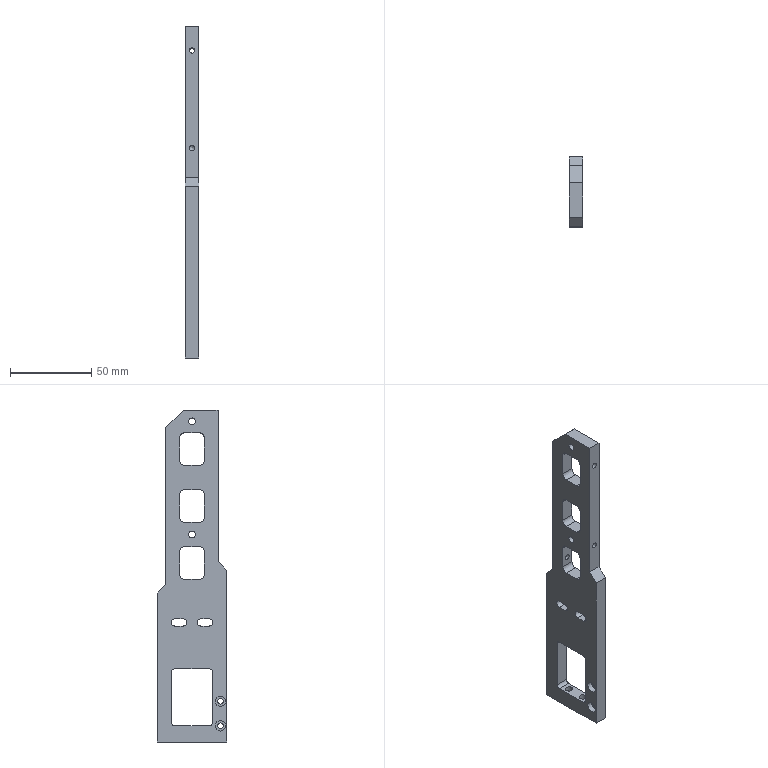CAM job | NX | 3+2 milling, drilling | part box 8 x 43 x 204 mm | stock box 10 x 45 x 209 mm
Tools:
number,name,description,diameter,corner_radius,flute_length,length,flutes
3,D3,平底铣刀-粗,3.0,0.0,20.0,75.0,2
4,D4,平底铣刀-粗,4.0,0.0,25.0,75.0,2
9,D10,平底铣刀-粗,10.0,0.0,35.0,75.0,2
17,D3-J,平底铣刀-精,3.0,0.0,50.0,75.0,2
7,D6-J,平底铣刀-精,6.0,0.0,25.0,75.0,2
1,D80R0.8_FACEMILL,圆鼻刀-粗,80.0,0.8,50.0,75.0,2
1,D80R0.8_FACEMILL-J,圆鼻刀-精,80.0,0.8,50.0,75.0,2
2,D6_CHAMFERMILL,倒角刀,6.0,0.0,3.0,25.0,2
22,M5X0.8,丝锥,4.2,0.0,35.0,50.0,2
13,ZT3.4,钻头,3.4,0.0,35.0,50.0,2
14,DRILL_4.2,Twist Drill 4.2 mm,4.2,0.0,41.0,41.738,2
Operations:
program,operation,operation_type,tool,method,geometry_group,spindle_rpm,surface_speed,feed_per_tooth,feed_cut,feed_plunge,cut_length_mm,path_length_mm,cut_time_min,machine_time_min
B,DYNROUGHD10_COPY,CavityMilling,D10,DYNROUGH-DEPTHK-STEPK,W-B,8000.0,251.32,0.25,4000.0,100.0,20829.161,20864.961,5.207,5.211
B,FLOORFACEONEPASS_COPY,VolumeBased25DMillingOperation,D80R0.8_FACEMILL-J,SIDEFINISH-DEPTHK-STEPG,W-B,4000.0,1005.28,0.125,1000.0,100.0,311.998,347.998,0.312,0.3156
B,C0.3CLOSEDCHAMFER6X45L_COPY,PlanarMilling,D6_CHAMFERMILL,CLIMBCHAMFER-DEPTH0-STEPG,W-B,7000.0,131.0,0.1071,1500.0,100.0,125.401,161.401,0.0836,0.0872
B,DRILLCHAMFER_1,Operation,D6_CHAMFERMILL,METHOD,W-B,8000.0,150.796,0.0625,1000.0,0.0,10.0,78.297,0.01,0.0168
B,DRILLCHAMFER_2,Operation,D6_CHAMFERMILL,METHOD,W-B,8000.0,150.796,0.0625,1000.0,0.0,11.4,135.365,0.0114,0.0238
B,C0.3FACEDEBURR6X45L__COPY,SurfaceContour,D6_CHAMFERMILL,CLIMBCHAMFER-DEPTH0-STEPG,W-B,8000.0,150.796,0.0938,1500.0,90.0,881.185,1357.684,0.5891,0.6367
A,TOPFACE,FaceMilling,D80R0.8_FACEMILL,SIDEFINISH-DEPTHK-STEPG,W-A,4000.0,1005.31,0.125,1000.0,100.0,298.0,334.0,0.298,0.3016
A,CONTOURROUGH_2,VolumeBased25DMillingOperation,D10,METHOD,W-A,8000.0,251.327,0.3125,5000.0,80.0,6157.638,6204.238,1.232,1.236
A,POCKETROUGH_1,VolumeBased25DMillingOperation,D10,METHOD,W-A,6000.0,188.0,0.25,4000.0,80.0,1427.126,1473.426,0.3568,0.3614
A,SLOTROUGH_1,VolumeBased25DMillingOperation,D10,METHOD,W-A,6000.0,113.0,0.2083,2500.0,100.0,1581.518,1792.018,0.6326,0.6537
A,SPOTDRILL-DEPTH0.8,Operation,D6_CHAMFERMILL,NONE,W-A,8000.0,150.796,0.0312,500.0,90.0,7.2,245.929,0.0144,0.0383
A,CBORE-DRILL0,Operation,ZT3.4,NONE,W-A,2800.0,29.908,0.0179,100.0,90.0,24.043,104.119,0.2404,0.2484
A,THRUHOLE-M5TAPDRILL,Operation,DRILL_4.2,NONE,W-A,3000.0,39.584,0.0583,350.0,90.0,32.524,175.554,0.0929,0.1072
A,THRUSLOTROUGH_1,VolumeBased25DMillingOperation,D3,METHOD,W-A,6000.0,75.398,0.1,1200.0,100.0,1721.352,1830.852,1.435,1.445
A,HOLEROUGHD4_1,CylinderMilling,D4,NONE,W-A,8000.0,100.531,0.075,1200.0,100.0,209.706,310.506,0.1748,0.1848
A,HOLEFINISHD4_1,CylinderMilling,D4,FINISHSTEPDEPTHOFF,W-A,8000.0,100.531,0.0312,500.0,100.0,37.912,138.712,0.0758,0.0859
A,POCKETFINISH_1,VolumeBased25DMillingOperation,D6-J,METHOD,W-A,6000.0,113.0,0.0833,1000.0,100.0,100.842,155.442,0.1008,0.1063
A,SLOTFINISH_1,VolumeBased25DMillingOperation,D6-J,METHOD,W-A,6000.0,113.0,0.0667,600.0,100.0,144.685,379.317,0.2411,0.2646
A,CORNERCLEAND4,ZLevelMilling,D3-J,METHOD,W-A,6000.0,75.0,0.25,2500.0,80.0,5162.849,5804.479,2.067,2.131
A,SLOTFINISH_2,VolumeBased25DMillingOperation,D3-J,METHOD,W-A,6000.0,56.549,0.05,600.0,100.0,67.763,217.463,0.1129,0.1279
A,CONTOURSIDE,ZLevelMilling,D3-J,METHOD,W-A,9000.0,84.823,0.1389,2500.0,80.0,345.025,478.484,0.1382,0.1515
A,SELECTEDBODYONLY,SurfaceContour,D6_CHAMFERMILL,METHOD,W-A,8000.0,150.796,0.1875,3000.0,100.0,863.851,1412.173,0.288,0.3428
A,MILLCHAMFER_1,PlanarMilling,D6_CHAMFERMILL,METHOD,W-A,8000.0,150.796,0.0312,500.0,100.0,36.041,187.555,0.0721,0.0872
A,MILLCHAMFER_2,PlanarMilling,D6_CHAMFERMILL,NONE,W-A,8000.0,150.796,0.0312,500.0,100.0,58.511,140.994,0.117,0.1253
A,THRUHOLE-TAPM5,Operation,M5X0.8,METHOD,W-A,500.0,6.597,0.0008,0.8,90.0,25.0,160.507,31.25,31.264
A,CONTOURSEMI_2,VolumeBased25DMillingOperation,D6-J,METHOD,W-A,8000.0,251.327,0.0625,1000.0,100.0,504.913,560.113,0.5049,0.5104